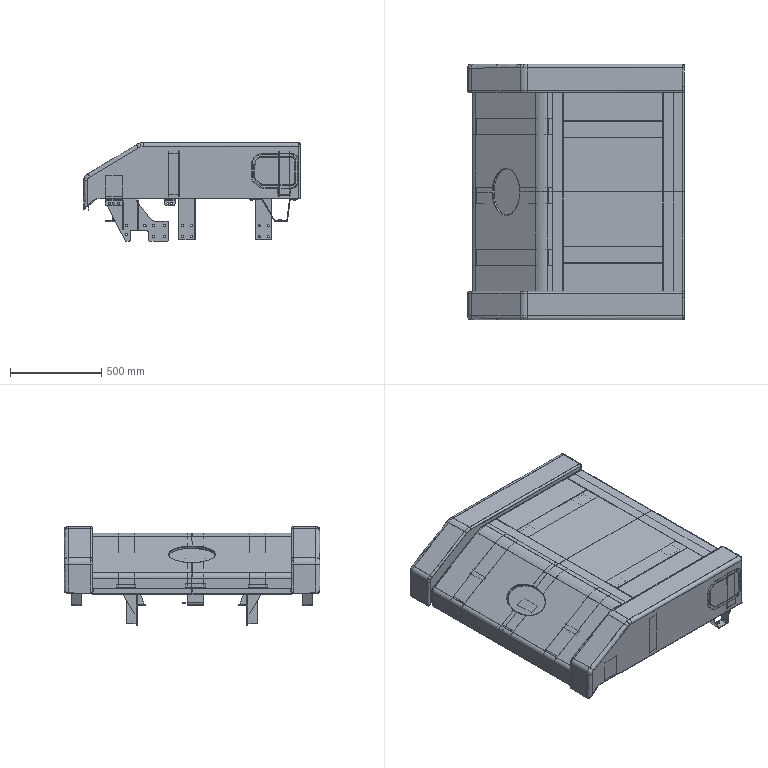Part | NX | features BREP 91 | 85 solids | 2183 faces | box 1184 x 1400 x 540.004 mm | volume 11251128 mm3 | plane 1218 | cylinder 571 | spline 226 | cone 168 | commonest cylinder face diameters 11 x120 13 x108 10 x56 8 x40 12 x38 20 x37